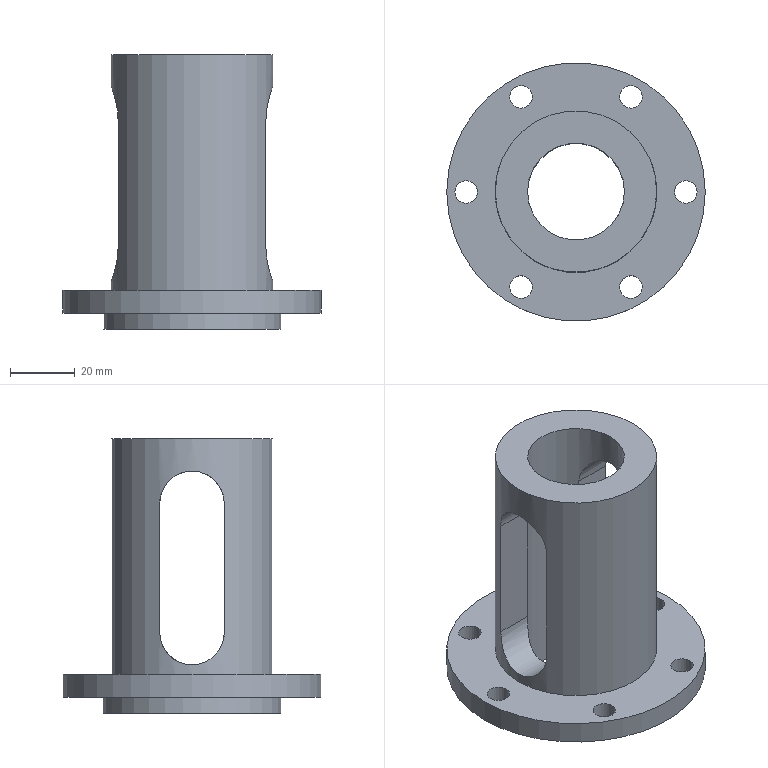NC program | NX | posted with a generic post | part box 80 x 80 x 85 mm
Lines 1 to 859 of 1822:
N10 G17 G21 G94 G90
(ZLEVEL_PROFILE , TOOL : D16R0.8)
N12 T04 M6
N14 G54
N16 G17 G0 G90 X-2. Y-34.454 B0. C0. S2200 M3
N18 G43 Z30. H4
N20 Z-12.694
N22 G94 G1 Y-65.21 Z-14.306 F1000.
N24 X-1.975 Y-65.3 Z-14.311
N26 X-1.922 Y-65.58 Z-14.326
N28 X-1.723 Y-66.033 Z-14.352
N30 X-1.419 Y-66.424 Z-14.378
N32 X-1.027 Y-66.727 Z-14.404
N34 X-0.846 Y-66.811 Z-14.414
N36 X-0.282 Y-66.98 F2200.
N38 G3 X0.282 Y-66.98 R1.984
N40 G1 X0.846 Y-66.811
N42 G3 X1.938 Y-65.488 R1.997
N44 G1 X1.978 Y-65.287
N46 X1.999 Y-65.009
N48 X2.
N50 Y-24.838
N52 X1.975 Y-24.7
N54 G3 X0.846 Y-23.188 R1.994
N56 G1 X0.282 Y-23.02
N58 G3 X-0.282 Y-23.02 R1.991
N60 G1 X-0.846 Y-23.188
N62 G3 X-1.975 Y-24.7 R1.989
N64 G1 X-1.979 Y-24.712
N66 X-2. Y-24.991
N68 Y-65.21
N70 X-1.975 Y-65.3
N72 X-1.959 Y-65.384
N74 G3 X-0.846 Y-66.811 R1.979
N76 G1 X-0.31 Y-66.971 Z-14.424
N78 X-0.032 Y-66.999 Z-14.429
N80 X0.248 Y-66.984 Z-14.434
N82 X0.517 Y-66.909 Z-14.439
N84 X0.786 Y-66.829 Z-14.444
N86 X1.037 Y-66.709 Z-14.449
N88 X1.266 Y-66.547 Z-14.453
N90 X1.47 Y-66.355 Z-14.458
N92 X1.644 Y-66.137 Z-14.463
N94 X1.787 Y-65.896 Z-14.468
N96 X1.894 Y-65.638 Z-14.473
N98 X1.962 Y-65.366 Z-14.478
N100 X1.993 Y-65.088 Z-14.483
N102 X2. Y-64.81 Z-14.488
N104 Y-56.407 Z-14.634
N106 Y-24.838
N108 X1.975 Y-24.7
N110 G3 X0.846 Y-23.188 R1.994
N112 G1 X0.282 Y-23.02
N114 G3 X-0.282 Y-23.02 R1.991
N116 G1 X-0.846 Y-23.188
N118 G3 X-1.975 Y-24.7 R1.989
N120 G1 X-1.979 Y-24.712
N122 X-2. Y-24.991
N124 Y-65.21
N126 X-1.975 Y-65.3
N128 X-1.959 Y-65.384
N130 G3 X-0.846 Y-66.811 R1.979
N132 G1 X-0.31 Y-66.971 Z-14.644
N134 X-0.032 Y-66.999 Z-14.649
N136 X0.248 Y-66.984 Z-14.654
N138 X0.517 Y-66.909 Z-14.659
N140 X0.786 Y-66.829 Z-14.664
N142 X1.037 Y-66.709 Z-14.669
N144 X1.266 Y-66.547 Z-14.673
N146 X1.47 Y-66.355 Z-14.678
N148 X1.644 Y-66.137 Z-14.683
N150 X1.787 Y-65.896 Z-14.688
N152 X1.894 Y-65.638 Z-14.693
N154 X1.962 Y-65.366 Z-14.698
N156 X1.993 Y-65.088 Z-14.703
N158 X2. Y-64.81 Z-14.708
N160 Y-56.407 Z-14.854
N162 Y-24.838
N164 X1.975 Y-24.7
N166 G3 X0.846 Y-23.188 R1.994
N168 G1 X0.282 Y-23.02
N170 G3 X-0.282 Y-23.02 R1.991
N172 G1 X-0.846 Y-23.188
N174 G3 X-1.975 Y-24.7 R1.989
N176 G1 X-1.979 Y-24.712
N178 X-2. Y-24.991
N180 Y-65.21
N182 X-1.975 Y-65.3
N184 X-1.959 Y-65.384
N186 G3 X-0.846 Y-66.811 R1.979
N188 G1 X-0.31 Y-66.971 Z-14.864
N190 X-0.032 Y-66.999 Z-14.869
N192 X0.248 Y-66.984 Z-14.874
N194 X0.517 Y-66.909 Z-14.879
N196 X0.786 Y-66.829 Z-14.884
N198 X1.037 Y-66.709 Z-14.889
N200 X1.266 Y-66.547 Z-14.893
N202 X1.47 Y-66.355 Z-14.898
N204 X1.644 Y-66.137 Z-14.903
N206 X1.787 Y-65.896 Z-14.908
N208 X1.894 Y-65.638 Z-14.913
N210 X1.962 Y-65.366 Z-14.918
N212 X1.993 Y-65.088 Z-14.923
N214 X2. Y-64.81 Z-14.928
N216 Y-56.407 Z-15.074
N218 Y-24.838
N220 X1.975 Y-24.7
N222 G3 X0.846 Y-23.188 R1.994
N224 G1 X0.282 Y-23.02
N226 G3 X-0.282 Y-23.02 R1.991
N228 G1 X-0.846 Y-23.188
N230 G3 X-1.975 Y-24.7 R1.989
N232 G1 X-1.979 Y-24.712
N234 X-2. Y-24.991
N236 Y-65.21
N238 X-1.975 Y-65.3
N240 X-1.959 Y-65.384
N242 G3 X-0.846 Y-66.811 R1.979
N244 G1 X-0.31 Y-66.971 Z-15.084
N246 X-0.032 Y-66.999 Z-15.089
N248 X0.248 Y-66.984 Z-15.094
N250 X0.517 Y-66.909 Z-15.099
N252 X0.786 Y-66.829 Z-15.104
N254 X1.037 Y-66.709 Z-15.109
N256 X1.266 Y-66.547 Z-15.113
N258 X1.47 Y-66.355 Z-15.118
N260 X1.644 Y-66.137 Z-15.123
N262 X1.787 Y-65.896 Z-15.128
N264 X1.894 Y-65.638 Z-15.133
N266 X1.962 Y-65.366 Z-15.138
N268 X1.993 Y-65.088 Z-15.143
N270 X2. Y-64.81 Z-15.148
N272 Y-56.407 Z-15.294
N274 Y-24.838
N276 X1.975 Y-24.7
N278 G3 X0.846 Y-23.188 R1.994
N280 G1 X0.282 Y-23.02
N282 G3 X-0.282 Y-23.02 R1.991
N284 G1 X-0.846 Y-23.188
N286 G3 X-1.975 Y-24.7 R1.989
N288 G1 X-1.979 Y-24.712
N290 X-2. Y-24.991
N292 Y-65.21
N294 X-1.975 Y-65.3
N296 X-1.959 Y-65.384
N298 G3 X-0.846 Y-66.811 R1.979
N300 G1 X-0.31 Y-66.971 Z-15.304
N302 X-0.032 Y-66.999 Z-15.309
N304 X0.248 Y-66.984 Z-15.314
N306 X0.517 Y-66.909 Z-15.319
N308 X0.786 Y-66.829 Z-15.324
N310 X1.037 Y-66.709 Z-15.329
N312 X1.266 Y-66.547 Z-15.333
N314 X1.47 Y-66.355 Z-15.338
N316 X1.644 Y-66.137 Z-15.343
N318 X1.787 Y-65.896 Z-15.348
N320 X1.894 Y-65.638 Z-15.353
N322 X1.962 Y-65.366 Z-15.358
N324 X1.993 Y-65.088 Z-15.363
N326 X2. Y-64.81 Z-15.368
N328 Y-56.407 Z-15.514
N330 Y-24.838
N332 X1.975 Y-24.7
N334 G3 X0.846 Y-23.188 R1.994
N336 G1 X0.282 Y-23.02
N338 G3 X-0.282 Y-23.02 R1.991
N340 G1 X-0.846 Y-23.188
N342 G3 X-1.975 Y-24.7 R1.989
N344 G1 X-1.979 Y-24.712
N346 X-2. Y-24.991
N348 Y-65.21
N350 X-1.975 Y-65.3
N352 X-1.959 Y-65.384
N354 G3 X-0.846 Y-66.811 R1.979
N356 G1 X-0.31 Y-66.971 Z-15.524
N358 X-0.032 Y-66.999 Z-15.529
N360 X0.248 Y-66.984 Z-15.534
N362 X0.517 Y-66.909 Z-15.539
N364 X0.786 Y-66.829 Z-15.544
N366 X1.037 Y-66.709 Z-15.549
N368 X1.266 Y-66.547 Z-15.553
N370 X1.47 Y-66.355 Z-15.558
N372 X1.644 Y-66.137 Z-15.563
N374 X1.787 Y-65.896 Z-15.568
N376 X1.894 Y-65.638 Z-15.573
N378 X1.962 Y-65.366 Z-15.578
N380 X1.993 Y-65.088 Z-15.583
N382 X2. Y-64.81 Z-15.588
N384 Y-56.407 Z-15.734
N386 Y-24.838
N388 X1.975 Y-24.7
N390 G3 X0.846 Y-23.188 R1.994
N392 G1 X0.282 Y-23.02
N394 G3 X-0.282 Y-23.02 R1.991
N396 G1 X-0.846 Y-23.188
N398 G3 X-1.975 Y-24.7 R1.989
N400 G1 X-1.979 Y-24.712
N402 X-2. Y-24.991
N404 Y-65.21
N406 X-1.975 Y-65.3
N408 X-1.959 Y-65.384
N410 G3 X-0.846 Y-66.811 R1.979
N412 G1 X-0.586 Y-66.912 Z-15.739
N414 X-0.313 Y-66.975 Z-15.744
N416 X-0.034 Y-67. Z-15.749
N418 X0.245 Y-66.985 Z-15.754
N420 X0.52 Y-66.931 Z-15.759
N422 X0.784 Y-66.84 Z-15.764
N424 X1.034 Y-66.712 Z-15.769
N426 X1.262 Y-66.551 Z-15.773
N428 X1.467 Y-66.36 Z-15.778
N430 X1.642 Y-66.142 Z-15.783
N432 X1.785 Y-65.901 Z-15.788
N434 X1.894 Y-65.643 Z-15.793
N436 X1.965 Y-65.373 Z-15.798
N438 X1.998 Y-65.095 Z-15.803
N440 X2. Y-64.815 Z-15.808
N442 Y-56.412 Z-15.954
N444 Y-25.
N446 G3 X0. Y-23. R2.
N448 X-2. Y-25. R2.
N450 G1 Y-65.
N452 G3 X-0.847 Y-66.812 R2.
N454 G1 X-0.621 Y-66.901 Z-15.959
N456 X-0.505 Y-66.935 Z-15.961
N458 X-0.445 Y-66.95 Z-15.962
N460 X-0.325 Y-66.973 Z-15.964
N462 X-0.098 Y-66.997 Z-15.968
N464 X0.016 Y-67. Z-15.97
N466 X0.084 Y-66.998 Z-15.971
N468 X0.221 Y-66.987 Z-15.974
N470 X0.444 Y-66.95 Z-15.977
N472 X0.553 Y-66.922 Z-15.979
N474 X0.62 Y-66.902 Z-15.981
N476 X0.751 Y-66.853 Z-15.983
N478 X0.955 Y-66.756 Z-15.987
N480 X1.053 Y-66.7 Z-15.989
N482 X1.111 Y-66.662 Z-15.99
N484 X1.224 Y-66.581 Z-15.993
N486 X1.391 Y-66.436 Z-15.996
N488 X1.468 Y-66.357 Z-15.998
N490 X1.516 Y-66.303 Z-16.
N492 X1.605 Y-66.19 Z-16.002
N494 X1.73 Y-66.003 Z-16.006
N496 X1.783 Y-65.904 Z-16.008
N498 X1.813 Y-65.841 Z-16.009
N500 X1.868 Y-65.712 Z-16.012
N502 X1.932 Y-65.517 Z-16.015
N504 X1.955 Y-65.418 Z-16.017
N506 X1.97 Y-65.339 Z-16.019
N508 X1.992 Y-65.18 Z-16.021
N510 X2. Y-64.906 Z-16.026
N512 Y-64.632 Z-16.031
N514 Y-56.412 Z-16.174
N516 Y-25.
N518 G3 X0. Y-23. R2.
N520 X-2. Y-25. R2.
N522 G1 Y-65.
N524 G3 X-0.847 Y-66.812 R2.
N526 G1 X-0.621 Y-66.901 Z-16.179
N528 X-0.505 Y-66.935 Z-16.181
N530 X-0.445 Y-66.95 Z-16.182
N532 X-0.325 Y-66.973 Z-16.184
N534 X-0.098 Y-66.997 Z-16.188
N536 X0.016 Y-67. Z-16.19
N538 X0.084 Y-66.998 Z-16.191
N540 X0.221 Y-66.987 Z-16.194
N542 X0.444 Y-66.95 Z-16.197
N544 X0.553 Y-66.922 Z-16.199
N546 X0.62 Y-66.902 Z-16.201
N548 X0.751 Y-66.853 Z-16.203
N550 X0.955 Y-66.756 Z-16.207
N552 X1.053 Y-66.7 Z-16.209
N554 X1.111 Y-66.662 Z-16.21
N556 X1.224 Y-66.581 Z-16.213
N558 X1.391 Y-66.436 Z-16.216
N560 X1.468 Y-66.357 Z-16.218
N562 X1.516 Y-66.303 Z-16.22
N564 X1.605 Y-66.19 Z-16.222
N566 X1.73 Y-66.003 Z-16.226
N568 X1.783 Y-65.904 Z-16.228
N570 X1.813 Y-65.841 Z-16.229
N572 X1.868 Y-65.712 Z-16.232
N574 X1.932 Y-65.517 Z-16.235
N576 X1.955 Y-65.418 Z-16.237
N578 X1.97 Y-65.339 Z-16.239
N580 X1.992 Y-65.18 Z-16.241
N582 X2. Y-64.906 Z-16.246
N584 Y-64.632 Z-16.251
N586 Y-56.412 Z-16.394
N588 Y-25.
N590 G3 X0. Y-23. R2.
N592 X-2. Y-25. R2.
N594 G1 Y-65.
N596 G3 X-0.847 Y-66.812 R2.
N598 G1 X-0.621 Y-66.901 Z-16.399
N600 X-0.505 Y-66.935 Z-16.401
N602 X-0.445 Y-66.95 Z-16.402
N604 X-0.325 Y-66.973 Z-16.404
N606 X-0.098 Y-66.997 Z-16.408
N608 X0.016 Y-67. Z-16.41
N610 X0.084 Y-66.998 Z-16.411
N612 X0.221 Y-66.987 Z-16.414
N614 X0.444 Y-66.95 Z-16.417
N616 X0.553 Y-66.922 Z-16.419
N618 X0.62 Y-66.902 Z-16.421
N620 X0.751 Y-66.853 Z-16.423
N622 X0.955 Y-66.756 Z-16.427
N624 X1.053 Y-66.7 Z-16.429
N626 X1.111 Y-66.662 Z-16.43
N628 X1.224 Y-66.581 Z-16.433
N630 X1.391 Y-66.436 Z-16.436
N632 X1.468 Y-66.357 Z-16.438
N634 X1.516 Y-66.303 Z-16.44
N636 X1.605 Y-66.19 Z-16.442
N638 X1.73 Y-66.003 Z-16.446
N640 X1.783 Y-65.904 Z-16.448
N642 X1.813 Y-65.841 Z-16.449
N644 X1.868 Y-65.712 Z-16.452
N646 X1.932 Y-65.517 Z-16.455
N648 X1.955 Y-65.418 Z-16.457
N650 X1.97 Y-65.339 Z-16.459
N652 X1.992 Y-65.18 Z-16.461
N654 X2. Y-64.906 Z-16.466
N656 Y-64.632 Z-16.471
N658 Y-56.412 Z-16.614
N660 Y-25.
N662 G3 X0. Y-23. R2.
N664 X-2. Y-25. R2.
N666 G1 Y-65.
N668 G3 X-0.847 Y-66.812 R2.
N670 G1 X-0.621 Y-66.901 Z-16.619
N672 X-0.505 Y-66.935 Z-16.621
N674 X-0.445 Y-66.95 Z-16.622
N676 X-0.325 Y-66.973 Z-16.624
N678 X-0.098 Y-66.997 Z-16.628
N680 X0.016 Y-67. Z-16.63
N682 X0.084 Y-66.998 Z-16.631
N684 X0.221 Y-66.987 Z-16.634
N686 X0.444 Y-66.95 Z-16.637
N688 X0.553 Y-66.922 Z-16.639
N690 X0.62 Y-66.902 Z-16.641
N692 X0.751 Y-66.853 Z-16.643
N694 X0.955 Y-66.756 Z-16.647
N696 X1.053 Y-66.7 Z-16.649
N698 X1.111 Y-66.662 Z-16.65
N700 X1.224 Y-66.581 Z-16.653
N702 X1.391 Y-66.436 Z-16.656
N704 X1.468 Y-66.357 Z-16.658
N706 X1.516 Y-66.303 Z-16.66
N708 X1.605 Y-66.19 Z-16.662
N710 X1.73 Y-66.003 Z-16.666
N712 X1.783 Y-65.904 Z-16.668
N714 X1.813 Y-65.841 Z-16.669
N716 X1.868 Y-65.712 Z-16.672
N718 X1.932 Y-65.517 Z-16.675
N720 X1.955 Y-65.418 Z-16.677
N722 X1.97 Y-65.339 Z-16.679
N724 X1.992 Y-65.18 Z-16.681
N726 X2. Y-64.906 Z-16.686
N728 Y-64.632 Z-16.691
N730 Y-56.412 Z-16.834
N732 Y-25.
N734 G3 X0. Y-23. R2.
N736 X-2. Y-25. R2.
N738 G1 Y-65.
N740 G3 X-0.847 Y-66.812 R2.
N742 G1 X-0.621 Y-66.901 Z-16.839
N744 X-0.505 Y-66.935 Z-16.841
N746 X-0.445 Y-66.95 Z-16.842
N748 X-0.325 Y-66.973 Z-16.844
N750 X-0.098 Y-66.997 Z-16.848
N752 X0.016 Y-67. Z-16.85
N754 X0.084 Y-66.998 Z-16.851
N756 X0.221 Y-66.987 Z-16.854
N758 X0.444 Y-66.95 Z-16.857
N760 X0.553 Y-66.922 Z-16.859
N762 X0.62 Y-66.902 Z-16.861
N764 X0.751 Y-66.853 Z-16.863
N766 X0.955 Y-66.756 Z-16.867
N768 X1.053 Y-66.7 Z-16.869
N770 X1.111 Y-66.662 Z-16.87
N772 X1.224 Y-66.581 Z-16.873
N774 X1.391 Y-66.436 Z-16.876
N776 X1.468 Y-66.357 Z-16.878
N778 X1.516 Y-66.303 Z-16.88
N780 X1.605 Y-66.19 Z-16.882
N782 X1.73 Y-66.003 Z-16.886
N784 X1.783 Y-65.904 Z-16.888
N786 X1.813 Y-65.841 Z-16.889
N788 X1.868 Y-65.712 Z-16.892
N790 X1.932 Y-65.517 Z-16.895
N792 X1.955 Y-65.418 Z-16.897
N794 X1.97 Y-65.339 Z-16.899
N796 X1.992 Y-65.18 Z-16.901
N798 X2. Y-64.906 Z-16.906
N800 Y-64.632 Z-16.911
N802 Y-56.412 Z-17.054
N804 Y-25.
N806 G3 X0. Y-23. R2.
N808 X-2. Y-25. R2.
N810 G1 Y-65.
N812 G3 X-0.847 Y-66.812 R2.
N814 G1 X-0.621 Y-66.901 Z-17.059
N816 X-0.505 Y-66.935 Z-17.061
N818 X-0.445 Y-66.95 Z-17.062
N820 X-0.325 Y-66.973 Z-17.064
N822 X-0.098 Y-66.997 Z-17.068
N824 X0.016 Y-67. Z-17.07
N826 X0.084 Y-66.998 Z-17.071
N828 X0.221 Y-66.987 Z-17.074
N830 X0.444 Y-66.95 Z-17.077
N832 X0.553 Y-66.922 Z-17.079
N834 X0.62 Y-66.902 Z-17.081
N836 X0.751 Y-66.853 Z-17.083
N838 X0.955 Y-66.756 Z-17.087
N840 X1.053 Y-66.699 Z-17.089
N842 X1.111 Y-66.662 Z-17.09
N844 X1.224 Y-66.581 Z-17.093
N846 X1.391 Y-66.436 Z-17.096
N848 X1.468 Y-66.357 Z-17.098
N850 X1.516 Y-66.303 Z-17.1
N852 X1.605 Y-66.19 Z-17.102
N854 X1.73 Y-66.003 Z-17.106
N856 X1.783 Y-65.904 Z-17.108
N858 X1.813 Y-65.841 Z-17.109
N860 X1.868 Y-65.712 Z-17.112
N862 X1.932 Y-65.517 Z-17.115
N864 X1.955 Y-65.418 Z-17.117
N866 X1.97 Y-65.339 Z-17.119
N868 X1.992 Y-65.18 Z-17.121
N870 X2. Y-64.906 Z-17.126
N872 Y-64.632 Z-17.131
N874 Y-56.412 Z-17.274
N876 Y-25.
N878 G3 X0. Y-23. R2.
N880 X-2. Y-25. R2.
N882 G1 Y-65.
N884 G3 X-0.847 Y-66.812 R2.
N886 G1 X-0.621 Y-66.901 Z-17.279
N888 X-0.505 Y-66.935 Z-17.281
N890 X-0.445 Y-66.95 Z-17.282
N892 X-0.325 Y-66.973 Z-17.284
N894 X-0.098 Y-66.997 Z-17.288
N896 X0.016 Y-67. Z-17.29
N898 X0.084 Y-66.998 Z-17.291
N900 X0.221 Y-66.987 Z-17.294
N902 X0.444 Y-66.95 Z-17.297
N904 X0.553 Y-66.922 Z-17.299
N906 X0.62 Y-66.902 Z-17.301
N908 X0.751 Y-66.853 Z-17.303
N910 X0.955 Y-66.756 Z-17.307
N912 X1.053 Y-66.699 Z-17.309
N914 X1.111 Y-66.662 Z-17.31
N916 X1.224 Y-66.581 Z-17.313
N918 X1.391 Y-66.436 Z-17.316
N920 X1.468 Y-66.357 Z-17.318
N922 X1.516 Y-66.303 Z-17.32
N924 X1.605 Y-66.19 Z-17.322
N926 X1.73 Y-66.003 Z-17.326
N928 X1.783 Y-65.904 Z-17.328
N930 X1.813 Y-65.841 Z-17.329
N932 X1.868 Y-65.712 Z-17.332
N934 X1.932 Y-65.517 Z-17.335
N936 X1.955 Y-65.418 Z-17.337
N938 X1.97 Y-65.339 Z-17.339
N940 X1.992 Y-65.18 Z-17.341
N942 X2. Y-64.906 Z-17.346
N944 Y-64.632 Z-17.351
N946 Y-56.412 Z-17.494
N948 Y-25.
N950 G3 X0. Y-23. R2.
N952 X-2. Y-25. R2.
N954 G1 Y-65.
N956 G3 X-0.847 Y-66.812 R2.
N958 G1 X-0.621 Y-66.901 Z-17.499
N960 X-0.505 Y-66.935 Z-17.501
N962 X-0.445 Y-66.95 Z-17.502
N964 X-0.325 Y-66.973 Z-17.504
N966 X-0.098 Y-66.997 Z-17.508
N968 X0.016 Y-67. Z-17.51
N970 X0.084 Y-66.998 Z-17.511
N972 X0.221 Y-66.987 Z-17.514
N974 X0.444 Y-66.95 Z-17.517
N976 X0.553 Y-66.922 Z-17.519
N978 X0.62 Y-66.902 Z-17.521
N980 X0.751 Y-66.853 Z-17.523
N982 X0.955 Y-66.756 Z-17.527
N984 X1.053 Y-66.699 Z-17.529
N986 X1.111 Y-66.662 Z-17.53
N988 X1.224 Y-66.581 Z-17.533
N990 X1.391 Y-66.436 Z-17.536
N992 X1.468 Y-66.357 Z-17.538
N994 X1.516 Y-66.303 Z-17.54
N996 X1.605 Y-66.19 Z-17.542
N998 X1.73 Y-66.003 Z-17.546
N1000 X1.783 Y-65.904 Z-17.548
N1002 X1.813 Y-65.841 Z-17.549
N1004 X1.868 Y-65.712 Z-17.552
N1006 X1.932 Y-65.517 Z-17.555
N1008 X1.955 Y-65.418 Z-17.557
N1010 X1.97 Y-65.339 Z-17.559
N1012 X1.992 Y-65.18 Z-17.561
N1014 X2. Y-64.906 Z-17.566
N1016 Y-64.632 Z-17.571
N1018 Y-56.412 Z-17.714
N1020 Y-25.
N1022 G3 X0. Y-23. R2.
N1024 X-2. Y-25. R2.
N1026 G1 Y-65.
N1028 G3 X-0.847 Y-66.812 R2.
N1030 G1 X-0.621 Y-66.901 Z-17.719
N1032 X-0.505 Y-66.935 Z-17.721
N1034 X-0.445 Y-66.95 Z-17.722
N1036 X-0.325 Y-66.973 Z-17.724
N1038 X-0.098 Y-66.997 Z-17.728
N1040 X0.016 Y-67. Z-17.73
N1042 X0.084 Y-66.998 Z-17.731
N1044 X0.221 Y-66.987 Z-17.734
N1046 X0.444 Y-66.95 Z-17.737
N1048 X0.553 Y-66.922 Z-17.739
N1050 X0.62 Y-66.902 Z-17.741
N1052 X0.751 Y-66.853 Z-17.743
N1054 X0.955 Y-66.756 Z-17.747
N1056 X1.053 Y-66.699 Z-17.749
N1058 X1.111 Y-66.662 Z-17.75
N1060 X1.224 Y-66.581 Z-17.753
N1062 X1.391 Y-66.436 Z-17.756
N1064 X1.468 Y-66.357 Z-17.758
N1066 X1.516 Y-66.303 Z-17.76
N1068 X1.605 Y-66.19 Z-17.762
N1070 X1.73 Y-66.003 Z-17.766
N1072 X1.783 Y-65.904 Z-17.768
N1074 X1.813 Y-65.841 Z-17.769
N1076 X1.868 Y-65.712 Z-17.772
N1078 X1.932 Y-65.517 Z-17.775
N1080 X1.955 Y-65.418 Z-17.777
N1082 X1.97 Y-65.339 Z-17.779
N1084 X1.992 Y-65.18 Z-17.781
N1086 X2. Y-64.906 Z-17.786
N1088 Y-64.632 Z-17.791
N1090 Y-56.412 Z-17.934
N1092 Y-25.
N1094 G3 X0. Y-23. R2.
N1096 X-2. Y-25. R2.
N1098 G1 Y-65.
N1100 G3 X-0.847 Y-66.812 R2.
N1102 G1 X-0.621 Y-66.901 Z-17.939
N1104 X-0.505 Y-66.935 Z-17.941
N1106 X-0.445 Y-66.95 Z-17.942
N1108 X-0.325 Y-66.973 Z-17.944
N1110 X-0.098 Y-66.997 Z-17.948
N1112 X0.016 Y-67. Z-17.95
N1114 X0.084 Y-66.998 Z-17.951
N1116 X0.221 Y-66.987 Z-17.954
N1118 X0.444 Y-66.95 Z-17.957
N1120 X0.553 Y-66.922 Z-17.959
N1122 X0.62 Y-66.902 Z-17.961
N1124 X0.751 Y-66.853 Z-17.963
N1126 X0.955 Y-66.756 Z-17.967
N1128 X1.053 Y-66.699 Z-17.969
N1130 X1.111 Y-66.662 Z-17.97
N1132 X1.224 Y-66.581 Z-17.973
N1134 X1.391 Y-66.436 Z-17.976
N1136 X1.468 Y-66.357 Z-17.978
N1138 X1.516 Y-66.303 Z-17.98
N1140 X1.605 Y-66.19 Z-17.982
N1142 X1.73 Y-66.003 Z-17.986
N1144 X1.783 Y-65.905 Z-17.988
N1146 X1.813 Y-65.841 Z-17.989
N1148 X1.868 Y-65.712 Z-17.992
N1150 X1.932 Y-65.517 Z-17.995
N1152 X1.955 Y-65.418 Z-17.997
N1154 X1.97 Y-65.339 Z-17.999
N1156 X1.992 Y-65.18 Z-18.001
N1158 X2. Y-64.906 Z-18.006
N1160 Y-64.632 Z-18.011
N1162 Y-56.412 Z-18.154
N1164 Y-25.
N1166 G3 X0. Y-23. R2.
N1168 X-2. Y-25. R2.
N1170 G1 Y-65.
N1172 G3 X-0.847 Y-66.812 R2.
N1174 G1 X-0.621 Y-66.901 Z-18.159
N1176 X-0.505 Y-66.935 Z-18.161
N1178 X-0.445 Y-66.95 Z-18.162
N1180 X-0.325 Y-66.973 Z-18.164
N1182 X-0.098 Y-66.997 Z-18.168
N1184 X0.016 Y-67. Z-18.17
N1186 X0.084 Y-66.998 Z-18.171
N1188 X0.221 Y-66.987 Z-18.174
N1190 X0.444 Y-66.95 Z-18.177
N1192 X0.553 Y-66.922 Z-18.179
N1194 X0.62 Y-66.902 Z-18.181
N1196 X0.751 Y-66.853 Z-18.183
N1198 X0.955 Y-66.756 Z-18.187
N1200 X1.053 Y-66.699 Z-18.189
N1202 X1.111 Y-66.662 Z-18.19
N1204 X1.224 Y-66.581 Z-18.193
N1206 X1.391 Y-66.436 Z-18.196
N1208 X1.468 Y-66.357 Z-18.198
N1210 X1.516 Y-66.303 Z-18.2
N1212 X1.605 Y-66.19 Z-18.202
N1214 X1.73 Y-66.003 Z-18.206
N1216 X1.783 Y-65.905 Z-18.208
N1218 X1.813 Y-65.841 Z-18.209
N1220 X1.868 Y-65.712 Z-18.212
N1222 X1.932 Y-65.517 Z-18.215
N1224 X1.955 Y-65.418 Z-18.217
N1226 X1.97 Y-65.339 Z-18.219
N1228 X1.992 Y-65.18 Z-18.221
N1230 X2. Y-64.906 Z-18.226
N1232 Y-64.632 Z-18.231
N1234 Y-56.412 Z-18.374
N1236 Y-25.
N1238 G3 X0. Y-23. R2.
N1240 X-2. Y-25. R2.
N1242 G1 Y-65.
N1244 G3 X-0.847 Y-66.812 R2.
N1246 G1 X-0.621 Y-66.901 Z-18.379
N1248 X-0.505 Y-66.935 Z-18.381
N1250 X-0.445 Y-66.95 Z-18.382
N1252 X-0.325 Y-66.973 Z-18.384
N1254 X-0.098 Y-66.997 Z-18.388
N1256 X0.016 Y-67. Z-18.39
N1258 X0.084 Y-66.998 Z-18.391
N1260 X0.221 Y-66.987 Z-18.394
N1262 X0.444 Y-66.95 Z-18.397
N1264 X0.553 Y-66.922 Z-18.399
N1266 X0.62 Y-66.902 Z-18.401
N1268 X0.751 Y-66.853 Z-18.403
N1270 X0.955 Y-66.756 Z-18.407
N1272 X1.053 Y-66.699 Z-18.409
N1274 X1.111 Y-66.662 Z-18.41
N1276 X1.224 Y-66.581 Z-18.413
N1278 X1.391 Y-66.436 Z-18.416
N1280 X1.468 Y-66.357 Z-18.418
N1282 X1.516 Y-66.303 Z-18.42
N1284 X1.605 Y-66.19 Z-18.422
N1286 X1.73 Y-66.003 Z-18.426
N1288 X1.783 Y-65.905 Z-18.428
N1290 X1.813 Y-65.841 Z-18.429
N1292 X1.868 Y-65.712 Z-18.432
N1294 X1.931 Y-65.517 Z-18.435
N1296 X1.955 Y-65.418 Z-18.437
N1298 X1.97 Y-65.339 Z-18.439
N1300 X1.992 Y-65.18 Z-18.441
N1302 X2. Y-64.906 Z-18.446
N1304 Y-64.632 Z-18.451
N1306 Y-56.412 Z-18.594
N1308 Y-25.
N1310 G3 X0. Y-23. R2.
N1312 X-2. Y-25. R2.
N1314 G1 Y-65.
N1316 G3 X-0.847 Y-66.812 R2.
N1318 G1 X-0.621 Y-66.901 Z-18.599
N1320 X-0.505 Y-66.935 Z-18.601
N1322 X-0.445 Y-66.95 Z-18.602
N1324 X-0.325 Y-66.973 Z-18.604
N1326 X-0.098 Y-66.997 Z-18.608
N1328 X0.016 Y-67. Z-18.61
N1330 X0.084 Y-66.998 Z-18.611
N1332 X0.221 Y-66.987 Z-18.614
N1334 X0.444 Y-66.95 Z-18.617
N1336 X0.553 Y-66.922 Z-18.619
N1338 X0.62 Y-66.902 Z-18.621
N1340 X0.751 Y-66.853 Z-18.623
N1342 X0.955 Y-66.756 Z-18.627
N1344 X1.053 Y-66.699 Z-18.629
N1346 X1.111 Y-66.662 Z-18.63
N1348 X1.224 Y-66.581 Z-18.633
N1350 X1.391 Y-66.436 Z-18.636
N1352 X1.468 Y-66.357 Z-18.638
N1354 X1.516 Y-66.303 Z-18.64
N1356 X1.605 Y-66.19 Z-18.642
N1358 X1.73 Y-66.003 Z-18.646
N1360 X1.783 Y-65.905 Z-18.648
N1362 X1.813 Y-65.841 Z-18.649
N1364 X1.868 Y-65.712 Z-18.652
N1366 X1.931 Y-65.517 Z-18.655
N1368 X1.955 Y-65.418 Z-18.657
N1370 X1.97 Y-65.339 Z-18.659
N1372 X1.992 Y-65.18 Z-18.661
N1374 X2. Y-64.906 Z-18.666
N1376 Y-64.632 Z-18.671
N1378 Y-56.412 Z-18.814
N1380 Y-25.
N1382 G3 X0. Y-23. R2.
N1384 X-2. Y-25. R2.
N1386 G1 Y-65.
N1388 G3 X-0.847 Y-66.812 R2.
N1390 G1 X-0.621 Y-66.901 Z-18.819
N1392 X-0.505 Y-66.935 Z-18.821
N1394 X-0.445 Y-66.95 Z-18.822
N1396 X-0.325 Y-66.973 Z-18.824
N1398 X-0.098 Y-66.997 Z-18.828
N1400 X0.016 Y-67. Z-18.83
N1402 X0.084 Y-66.998 Z-18.831
N1404 X0.221 Y-66.987 Z-18.834
N1406 X0.444 Y-66.95 Z-18.837
N1408 X0.553 Y-66.922 Z-18.839
N1410 X0.62 Y-66.902 Z-18.841
N1412 X0.751 Y-66.853 Z-18.843
N1414 X0.955 Y-66.756 Z-18.847
N1416 X1.053 Y-66.699 Z-18.849
N1418 X1.111 Y-66.662 Z-18.85
N1420 X1.224 Y-66.581 Z-18.853
N1422 X1.391 Y-66.436 Z-18.856
N1424 X1.468 Y-66.357 Z-18.858
N1426 X1.516 Y-66.303 Z-18.86
N1428 X1.605 Y-66.19 Z-18.862
N1430 X1.73 Y-66.003 Z-18.866
N1432 X1.783 Y-65.905 Z-18.868
N1434 X1.813 Y-65.841 Z-18.869
N1436 X1.868 Y-65.712 Z-18.872
N1438 X1.931 Y-65.517 Z-18.875
N1440 X1.955 Y-65.418 Z-18.877
N1442 X1.97 Y-65.339 Z-18.879
N1444 X1.992 Y-65.18 Z-18.881
N1446 X2. Y-64.906 Z-18.886
N1448 Y-64.632 Z-18.891
N1450 Y-56.412 Z-19.034
N1452 Y-25.
N1454 G3 X0. Y-23. R2.
N1456 X-2. Y-25. R2.
N1458 G1 Y-65.
N1460 G3 X-0.847 Y-66.812 R2.
N1462 G1 X-0.621 Y-66.901 Z-19.039
N1464 X-0.505 Y-66.935 Z-19.041
N1466 X-0.445 Y-66.95 Z-19.042
N1468 X-0.325 Y-66.973 Z-19.044
N1470 X-0.098 Y-66.997 Z-19.048
N1472 X0.016 Y-67. Z-19.05
N1474 X0.084 Y-66.998 Z-19.051
N1476 X0.221 Y-66.987 Z-19.054
N1478 X0.444 Y-66.95 Z-19.057
N1480 X0.553 Y-66.922 Z-19.059
N1482 X0.62 Y-66.902 Z-19.061
N1484 X0.751 Y-66.853 Z-19.063
N1486 X0.955 Y-66.756 Z-19.067
N1488 X1.053 Y-66.699 Z-19.069
N1490 X1.111 Y-66.662 Z-19.07
N1492 X1.224 Y-66.581 Z-19.073
N1494 X1.391 Y-66.436 Z-19.076
N1496 X1.468 Y-66.357 Z-19.078
N1498 X1.516 Y-66.303 Z-19.08
N1500 X1.605 Y-66.19 Z-19.082
N1502 X1.73 Y-66.003 Z-19.086
N1504 X1.783 Y-65.905 Z-19.088
N1506 X1.813 Y-65.841 Z-19.089
N1508 X1.868 Y-65.712 Z-19.092
N1510 X1.931 Y-65.517 Z-19.095
N1512 X1.955 Y-65.418 Z-19.097
N1514 X1.97 Y-65.339 Z-19.099
N1516 X1.992 Y-65.18 Z-19.101
N1518 X2. Y-64.906 Z-19.106
N1520 Y-64.632 Z-19.111
N1522 Y-56.412 Z-19.254
N1524 Y-25.
N1526 G3 X0. Y-23. R2.
N1528 X-2. Y-25. R2.
N1530 G1 Y-65.
N1532 G3 X-0.847 Y-66.812 R2.
N1534 G1 X-0.621 Y-66.901 Z-19.259
N1536 X-0.505 Y-66.935 Z-19.261
N1538 X-0.445 Y-66.95 Z-19.262
N1540 X-0.325 Y-66.973 Z-19.264
N1542 X-0.098 Y-66.997 Z-19.268
N1544 X0.016 Y-67. Z-19.27
N1546 X0.084 Y-66.998 Z-19.271
N1548 X0.221 Y-66.987 Z-19.274
N1550 X0.444 Y-66.95 Z-19.277
N1552 X0.553 Y-66.922 Z-19.279
N1554 X0.62 Y-66.902 Z-19.281
N1556 X0.751 Y-66.853 Z-19.283
N1558 X0.955 Y-66.756 Z-19.287
N1560 X1.053 Y-66.699 Z-19.289
N1562 X1.111 Y-66.662 Z-19.29
N1564 X1.224 Y-66.581 Z-19.293
N1566 X1.391 Y-66.436 Z-19.296
N1568 X1.468 Y-66.357 Z-19.298
N1570 X1.515 Y-66.303 Z-19.3
N1572 X1.605 Y-66.19 Z-19.302
N1574 X1.73 Y-66.003 Z-19.306
N1576 X1.783 Y-65.905 Z-19.308
N1578 X1.813 Y-65.841 Z-19.309
N1580 X1.868 Y-65.712 Z-19.312
N1582 X1.931 Y-65.517 Z-19.315
N1584 X1.955 Y-65.418 Z-19.317
N1586 X1.97 Y-65.339 Z-19.319
N1588 X1.992 Y-65.18 Z-19.321
N1590 X2. Y-64.906 Z-19.326
N1592 Y-64.632 Z-19.331
N1594 Y-56.412 Z-19.474
N1596 Y-25.
N1598 G3 X0. Y-23. R2.
N1600 X-2. Y-25. R2.
N1602 G1 Y-65.
N1604 G3 X-0.847 Y-66.812 R2.
N1606 G1 X-0.621 Y-66.901 Z-19.479
N1608 X-0.505 Y-66.935 Z-19.481
N1610 X-0.445 Y-66.95 Z-19.482
N1612 X-0.325 Y-66.973 Z-19.484
N1614 X-0.098 Y-66.997 Z-19.488
N1616 X0.016 Y-67. Z-19.49
N1618 X0.084 Y-66.998 Z-19.491
N1620 X0.221 Y-66.987 Z-19.494
N1622 X0.444 Y-66.95 Z-19.497
N1624 X0.553 Y-66.922 Z-19.499
N1626 X0.62 Y-66.902 Z-19.501
N1628 X0.751 Y-66.853 Z-19.503
N1630 X0.955 Y-66.756 Z-19.507
N1632 X1.053 Y-66.699 Z-19.509
N1634 X1.111 Y-66.662 Z-19.51
N1636 X1.224 Y-66.581 Z-19.513
N1638 X1.391 Y-66.436 Z-19.516
N1640 X1.468 Y-66.357 Z-19.518
N1642 X1.515 Y-66.303 Z-19.52
N1644 X1.605 Y-66.19 Z-19.522
N1646 X1.73 Y-66.003 Z-19.526
N1648 X1.783 Y-65.905 Z-19.528
N1650 X1.813 Y-65.841 Z-19.529
N1652 X1.868 Y-65.712 Z-19.532
N1654 X1.931 Y-65.517 Z-19.535
N1656 X1.955 Y-65.418 Z-19.537
N1658 X1.97 Y-65.339 Z-19.539
N1660 X1.992 Y-65.18 Z-19.541
N1662 X2. Y-64.906 Z-19.546
N1664 Y-64.632 Z-19.551
N1666 Y-56.412 Z-19.694
N1668 Y-25.
N1670 G3 X0. Y-23. R2.
N1672 X-2. Y-25. R2.
N1674 G1 Y-65.
N1676 G3 X-0.847 Y-66.812 R2.
N1678 G1 X-0.621 Y-66.901 Z-19.699
N1680 X-0.505 Y-66.935 Z-19.701
N1682 X-0.445 Y-66.95 Z-19.702
N1684 X-0.325 Y-66.973 Z-19.704
N1686 X-0.098 Y-66.997 Z-19.708
N1688 X0.016 Y-67. Z-19.71
N1690 X0.084 Y-66.998 Z-19.711
N1692 X0.221 Y-66.987 Z-19.714
N1694 X0.444 Y-66.95 Z-19.717
N1696 X0.553 Y-66.922 Z-19.719
N1698 X0.62 Y-66.902 Z-19.721
N1700 X0.751 Y-66.853 Z-19.723
N1702 X0.955 Y-66.756 Z-19.727
N1704 X1.053 Y-66.699 Z-19.729
N1706 X1.111 Y-66.662 Z-19.73
N1708 X1.224 Y-66.581 Z-19.733
N1710 X1.391 Y-66.436 Z-19.736
N1712 X1.468 Y-66.357 Z-19.738
N1714 X1.515 Y-66.303 Z-19.74
N1716 X1.605 Y-66.19 Z-19.742